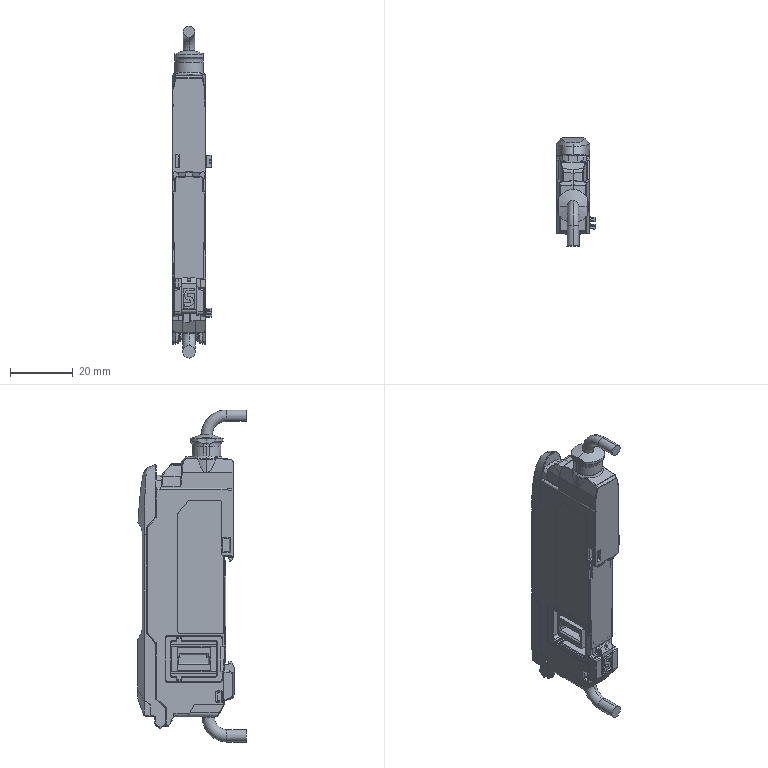Part | STEP file | [LR-XN11P]-Part-1 | 1 solid | 1090 faces | box 12.6 x 34.5 x 105.605 mm | volume 23912 mm3 | plane 589 | cylinder 294 | spline 153 | torus 20 | sphere 18 | cone 16 | commonest cylinder face diameters 0.4 x115 1 x37 0.6 x18 1.6 x15 2 x15 0.2 x10